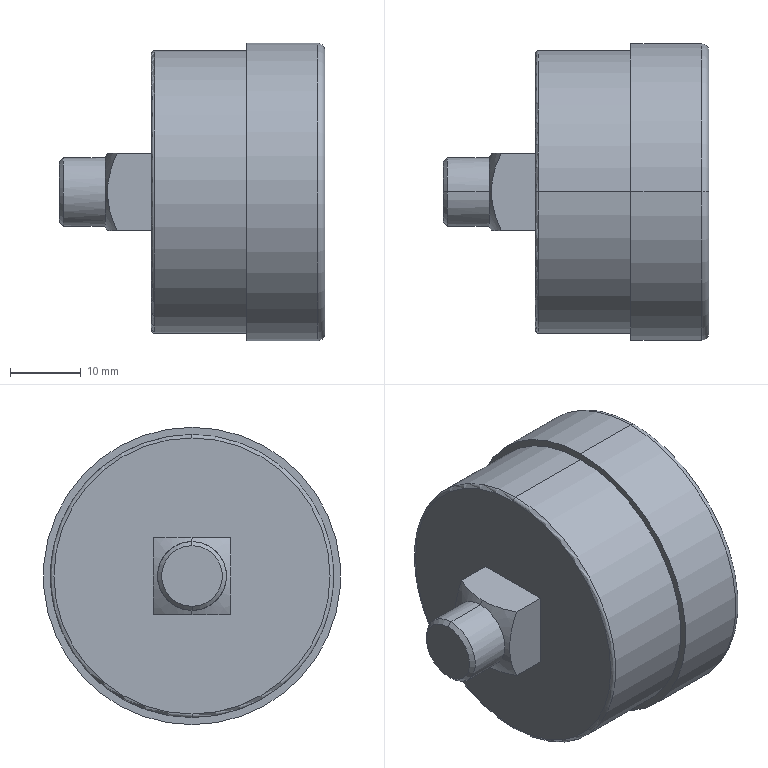Part | SolidWorks | features BaseBody 1 | 1 solid | 25 faces | box 37.5 x 42 x 42 mm | volume 32291 mm3 | plane 9 | cylinder 8 | torus 4 | cone 2 | spline 2 | commonest cylinder face diameters 9.728 x2 37.8 x2 40 x2 42 x2
STEP:
#1=CARTESIAN_POINT('',(-12.419,0.000000001,4.864));
#2=VERTEX_POINT('',#1);
#3=CARTESIAN_POINT('',(-12.419,-0.000000001,-4.864));
#4=VERTEX_POINT('',#3);
#5=CARTESIAN_POINT('',(-12.419,0.,0.));
#6=DIRECTION('',(1.,0.,0.));
#7=DIRECTION('',(0.,0.,-1.));
#8=AXIS2_PLACEMENT_3D('',#5,#6,#7);
#9=CIRCLE('',#8,4.864);
#10=EDGE_CURVE('',#2,#4,#9,.T.);
#11=ORIENTED_EDGE('',*,*,#10,.T.);
#12=CARTESIAN_POINT('',(-6.5,0.,-4.864));
#13=VERTEX_POINT('',#12);
#14=CARTESIAN_POINT('',(23.5,-0.000000004,-4.864));
#15=DIRECTION('',(1.,0.,0.));
#16=VECTOR('',#15,1000.);
#17=LINE('',#14,#16);
#18=EDGE_CURVE('',#4,#13,#17,.T.);
#19=ORIENTED_EDGE('',*,*,#18,.T.);
#20=CARTESIAN_POINT('',(-6.5,0.,4.864));
#21=VERTEX_POINT('',#20);
#22=CARTESIAN_POINT('',(-6.5,0.,4.864));
#23=CARTESIAN_POINT('',(-6.5,-2.547,4.864));
#24=CARTESIAN_POINT('',(-6.5,-5.09,3.281));
#25=CARTESIAN_POINT('',(-6.5,-6.402,0.));
#26=CARTESIAN_POINT('',(-6.5,-5.09,-3.281));
#27=CARTESIAN_POINT('',(-6.5,-2.547,-4.864));
#28=CARTESIAN_POINT('',(-6.5,0.,-4.864));
#29=B_SPLINE_CURVE_WITH_KNOTS('',6,(#22,#23,#24,#25,#26,#27,#28),.UNSPECIFIED.,.F.,.F.,(7,7),(0.,1.),.UNSPECIFIED.);
#30=EDGE_CURVE('',#21,#13,#29,.T.);
#31=ORIENTED_EDGE('',*,*,#30,.F.);
#32=CARTESIAN_POINT('',(23.5,0.000000004,4.864));
#33=DIRECTION('',(1.,0.,0.));
#34=VECTOR('',#33,1000.);
#35=LINE('',#32,#34);
#36=EDGE_CURVE('',#2,#21,#35,.T.);
#37=ORIENTED_EDGE('',*,*,#36,.F.);
#38=EDGE_LOOP('',(#11,#19,#31,#37));
#39=FACE_OUTER_BOUND('',#38,.T.);
#40=CARTESIAN_POINT('',(23.5,0.,0.));
#41=DIRECTION('',(1.,0.,0.));
#42=DIRECTION('',(0.,0.000000001,1.));
#43=AXIS2_PLACEMENT_3D('',#40,#41,#42);
#44=CYLINDRICAL_SURFACE('',#43,4.864);
#45=ADVANCED_FACE('',(#39),#44,.T.);
#46=CARTESIAN_POINT('',(-13.,0.000000001,4.283));
#47=VERTEX_POINT('',#46);
#48=CARTESIAN_POINT('',(-13.,-0.000000001,-4.283));
#49=VERTEX_POINT('',#48);
#50=CARTESIAN_POINT('',(-13.,0.,0.));
#51=DIRECTION('',(1.,0.,0.));
#52=DIRECTION('',(0.,0.,-1.));
#53=AXIS2_PLACEMENT_3D('',#50,#51,#52);
#54=CIRCLE('',#53,4.283);
#55=EDGE_CURVE('',#47,#49,#54,.T.);
#56=ORIENTED_EDGE('',*,*,#55,.T.);
#57=CARTESIAN_POINT('',(-12.419,-0.000000001,-4.864));
#58=DIRECTION('',(0.7071,0.,-0.7071));
#59=VECTOR('',#58,1000.);
#60=LINE('',#57,#59);
#61=EDGE_CURVE('',#49,#4,#60,.T.);
#62=ORIENTED_EDGE('',*,*,#61,.T.);
#63=ORIENTED_EDGE('',*,*,#10,.F.);
#64=CARTESIAN_POINT('',(-12.419,0.000000001,4.864));
#65=DIRECTION('',(0.7071,0.,0.7071));
#66=VECTOR('',#65,1000.);
#67=LINE('',#64,#66);
#68=EDGE_CURVE('',#47,#2,#67,.T.);
#69=ORIENTED_EDGE('',*,*,#68,.F.);
#70=EDGE_LOOP('',(#56,#62,#63,#69));
#71=FACE_OUTER_BOUND('',#70,.T.);
#72=CARTESIAN_POINT('',(-12.419,0.,0.));
#73=DIRECTION('',(1.,0.,0.));
#74=DIRECTION('',(0.,0.,1.));
#75=AXIS2_PLACEMENT_3D('',#72,#73,#74);
#76=CONICAL_SURFACE('',#75,4.864,0.7854);
#77=ADVANCED_FACE('',(#71),#76,.T.);
#78=CARTESIAN_POINT('',(23.5,0.,-18.9));
#79=VERTEX_POINT('',#78);
#80=CARTESIAN_POINT('',(23.5,-0.000000022,18.9));
#81=VERTEX_POINT('',#80);
#82=CARTESIAN_POINT('',(23.5,0.,0.));
#83=DIRECTION('',(1.,0.,0.));
#84=DIRECTION('',(0.,-0.000000001,1.));
#85=AXIS2_PLACEMENT_3D('',#82,#83,#84);
#86=CIRCLE('',#85,18.9);
#87=EDGE_CURVE('',#79,#81,#86,.T.);
#88=ORIENTED_EDGE('',*,*,#87,.F.);
#89=CARTESIAN_POINT('',(24.5,0.,-18.9));
#90=VERTEX_POINT('',#89);
#91=CARTESIAN_POINT('',(23.5,0.,-18.9));
#92=DIRECTION('',(1.,0.,0.));
#93=VECTOR('',#92,1000.);
#94=LINE('',#91,#93);
#95=EDGE_CURVE('',#79,#90,#94,.T.);
#96=ORIENTED_EDGE('',*,*,#95,.T.);
#97=CARTESIAN_POINT('',(24.5,0.,18.9));
#98=VERTEX_POINT('',#97);
#99=CARTESIAN_POINT('',(24.5,0.,0.));
#100=DIRECTION('',(1.,0.,0.));
#101=DIRECTION('',(0.,0.,-1.));
#102=AXIS2_PLACEMENT_3D('',#99,#100,#101);
#103=CIRCLE('',#102,18.9);
#104=EDGE_CURVE('',#90,#98,#103,.T.);
#105=ORIENTED_EDGE('',*,*,#104,.T.);
#106=CARTESIAN_POINT('',(23.5,0.,18.9));
#107=DIRECTION('',(1.,0.,0.));
#108=VECTOR('',#107,1000.);
#109=LINE('',#106,#108);
#110=EDGE_CURVE('',#81,#98,#109,.T.);
#111=ORIENTED_EDGE('',*,*,#110,.F.);
#112=EDGE_LOOP('',(#88,#96,#105,#111));
#113=FACE_OUTER_BOUND('',#112,.T.);
#114=CARTESIAN_POINT('',(23.5,0.,0.));
#115=DIRECTION('',(1.,0.,0.));
#116=DIRECTION('',(0.,0.,1.));
#117=AXIS2_PLACEMENT_3D('',#114,#115,#116);
#118=CYLINDRICAL_SURFACE('',#117,18.9);
#119=ADVANCED_FACE('',(#113),#118,.F.);
#120=CARTESIAN_POINT('',(23.5,0.000000004,21.));
#121=VERTEX_POINT('',#120);
#122=CARTESIAN_POINT('',(23.5,-0.000000004,-21.));
#123=VERTEX_POINT('',#122);
#124=CARTESIAN_POINT('',(23.5,0.,0.));
#125=DIRECTION('',(1.,0.,0.));
#126=DIRECTION('',(0.,0.,-1.));
#127=AXIS2_PLACEMENT_3D('',#124,#125,#126);
#128=CIRCLE('',#127,21.);
#129=EDGE_CURVE('',#121,#123,#128,.T.);
#130=ORIENTED_EDGE('',*,*,#129,.T.);
#131=CARTESIAN_POINT('',(24.5,-0.000000004,-20.));
#132=VERTEX_POINT('',#131);
#133=CARTESIAN_POINT('',(23.5,-0.000000004,-20.));
#134=DIRECTION('',(0.,-1.,0.));
#135=DIRECTION('',(0.,0.,-1.));
#136=AXIS2_PLACEMENT_3D('',#133,#134,#135);
#137=CIRCLE('',#136,1.);
#138=EDGE_CURVE('',#123,#132,#137,.T.);
#139=ORIENTED_EDGE('',*,*,#138,.T.);
#140=CARTESIAN_POINT('',(24.5,0.,20.));
#141=VERTEX_POINT('',#140);
#142=CARTESIAN_POINT('',(24.5,0.,0.));
#143=DIRECTION('',(1.,0.,0.));
#144=DIRECTION('',(0.,0.,1.));
#145=AXIS2_PLACEMENT_3D('',#142,#143,#144);
#146=CIRCLE('',#145,20.);
#147=EDGE_CURVE('',#141,#132,#146,.T.);
#148=ORIENTED_EDGE('',*,*,#147,.F.);
#149=CARTESIAN_POINT('',(23.5,0.000000004,20.));
#150=DIRECTION('',(0.,1.,0.));
#151=DIRECTION('',(0.,0.,1.));
#152=AXIS2_PLACEMENT_3D('',#149,#150,#151);
#153=CIRCLE('',#152,1.);
#154=EDGE_CURVE('',#121,#141,#153,.T.);
#155=ORIENTED_EDGE('',*,*,#154,.F.);
#156=EDGE_LOOP('',(#130,#139,#148,#155));
#157=FACE_OUTER_BOUND('',#156,.T.);
#158=CARTESIAN_POINT('',(23.5,0.,0.));
#159=DIRECTION('',(1.,0.,0.));
#160=DIRECTION('',(0.,0.,1.));
#161=AXIS2_PLACEMENT_3D('',#158,#159,#160);
#162=TOROIDAL_SURFACE('',#161,20.,1.);
#163=ADVANCED_FACE('',(#157),#162,.T.);
#164=CARTESIAN_POINT('',(13.5,0.000000004,21.));
#165=VERTEX_POINT('',#164);
#166=CARTESIAN_POINT('',(13.5,-0.000000004,-21.));
#167=VERTEX_POINT('',#166);
#168=CARTESIAN_POINT('',(13.5,0.,0.));
#169=DIRECTION('',(1.,0.,0.));
#170=DIRECTION('',(0.,0.,-1.));
#171=AXIS2_PLACEMENT_3D('',#168,#169,#170);
#172=CIRCLE('',#171,21.);
#173=EDGE_CURVE('',#165,#167,#172,.T.);
#174=ORIENTED_EDGE('',*,*,#173,.T.);
#175=CARTESIAN_POINT('',(23.5,-0.000000004,-21.));
#176=DIRECTION('',(1.,0.,0.));
#177=VECTOR('',#176,1000.);
#178=LINE('',#175,#177);
#179=EDGE_CURVE('',#167,#123,#178,.T.);
#180=ORIENTED_EDGE('',*,*,#179,.T.);
#181=ORIENTED_EDGE('',*,*,#129,.F.);
#182=CARTESIAN_POINT('',(23.5,0.000000004,21.));
#183=DIRECTION('',(1.,0.,0.));
#184=VECTOR('',#183,1000.);
#185=LINE('',#182,#184);
#186=EDGE_CURVE('',#165,#121,#185,.T.);
#187=ORIENTED_EDGE('',*,*,#186,.F.);
#188=EDGE_LOOP('',(#174,#180,#181,#187));
#189=FACE_OUTER_BOUND('',#188,.T.);
#190=CARTESIAN_POINT('',(23.5,0.,0.));
#191=DIRECTION('',(1.,0.,0.));
#192=DIRECTION('',(0.,0.,1.));
#193=AXIS2_PLACEMENT_3D('',#190,#191,#192);
#194=CYLINDRICAL_SURFACE('',#193,21.);
#195=ADVANCED_FACE('',(#189),#194,.T.);
#196=CARTESIAN_POINT('',(0.5,0.000000023,20.));
#197=VERTEX_POINT('',#196);
#198=CARTESIAN_POINT('',(0.5,-0.000000023,-20.));
#199=VERTEX_POINT('',#198);
#200=CARTESIAN_POINT('',(0.5,0.,0.));
#201=DIRECTION('',(1.,0.,0.));
#202=DIRECTION('',(0.,0.,-1.));
#203=AXIS2_PLACEMENT_3D('',#200,#201,#202);
#204=CIRCLE('',#203,20.);
#205=EDGE_CURVE('',#197,#199,#204,.T.);
#206=ORIENTED_EDGE('',*,*,#205,.T.);
#207=CARTESIAN_POINT('',(13.5,-0.000000015,-20.));
#208=VERTEX_POINT('',#207);
#209=CARTESIAN_POINT('',(23.5,-0.000000015,-20.));
#210=DIRECTION('',(1.,0.,0.));
#211=VECTOR('',#210,1000.);
#212=LINE('',#209,#211);
#213=EDGE_CURVE('',#199,#208,#212,.T.);
#214=ORIENTED_EDGE('',*,*,#213,.T.);
#215=CARTESIAN_POINT('',(13.5,0.,20.));
#216=VERTEX_POINT('',#215);
#217=CARTESIAN_POINT('',(13.5,0.,0.));
#218=DIRECTION('',(1.,0.,0.));
#219=DIRECTION('',(0.,0.,1.));
#220=AXIS2_PLACEMENT_3D('',#217,#218,#219);
#221=CIRCLE('',#220,20.);
#222=EDGE_CURVE('',#216,#208,#221,.T.);
#223=ORIENTED_EDGE('',*,*,#222,.F.);
#224=CARTESIAN_POINT('',(23.5,0.000000015,20.));
#225=DIRECTION('',(1.,0.,0.));
#226=VECTOR('',#225,1000.);
#227=LINE('',#224,#226);
#228=EDGE_CURVE('',#197,#216,#227,.T.);
#229=ORIENTED_EDGE('',*,*,#228,.F.);
#230=EDGE_LOOP('',(#206,#214,#223,#229));
#231=FACE_OUTER_BOUND('',#230,.T.);
#232=CARTESIAN_POINT('',(23.5,0.,0.));
#233=DIRECTION('',(1.,0.,0.));
#234=DIRECTION('',(0.,0.000000001,1.));
#235=AXIS2_PLACEMENT_3D('',#232,#233,#234);
#236=CYLINDRICAL_SURFACE('',#235,20.);
#237=ADVANCED_FACE('',(#231),#236,.T.);
#238=CARTESIAN_POINT('',(0.,0.000000023,19.5));
#239=VERTEX_POINT('',#238);
#240=CARTESIAN_POINT('',(0.,-0.000000023,-19.5));
#241=VERTEX_POINT('',#240);
#242=CARTESIAN_POINT('',(0.,0.,0.));
#243=DIRECTION('',(1.,0.,0.));
#244=DIRECTION('',(0.,0.,-1.));
#245=AXIS2_PLACEMENT_3D('',#242,#243,#244);
#246=CIRCLE('',#245,19.5);
#247=EDGE_CURVE('',#239,#241,#246,.T.);
#248=ORIENTED_EDGE('',*,*,#247,.T.);
#249=CARTESIAN_POINT('',(0.5,-0.000000023,-19.5));
#250=DIRECTION('',(0.,-1.,0.000000001));
#251=DIRECTION('',(0.,-0.000000001,-1.));
#252=AXIS2_PLACEMENT_3D('',#249,#250,#251);
#253=CIRCLE('',#252,0.5);
#254=EDGE_CURVE('',#241,#199,#253,.T.);
#255=ORIENTED_EDGE('',*,*,#254,.T.);
#256=ORIENTED_EDGE('',*,*,#205,.F.);
#257=CARTESIAN_POINT('',(0.5,0.000000023,19.5));
#258=DIRECTION('',(0.,1.,-0.000000001));
#259=DIRECTION('',(0.,0.000000001,1.));
#260=AXIS2_PLACEMENT_3D('',#257,#258,#259);
#261=CIRCLE('',#260,0.5);
#262=EDGE_CURVE('',#239,#197,#261,.T.);
#263=ORIENTED_EDGE('',*,*,#262,.F.);
#264=EDGE_LOOP('',(#248,#255,#256,#263));
#265=FACE_OUTER_BOUND('',#264,.T.);
#266=CARTESIAN_POINT('',(0.5,0.,0.));
#267=DIRECTION('',(1.,0.,0.));
#268=DIRECTION('',(0.,0.000000001,1.));
#269=AXIS2_PLACEMENT_3D('',#266,#267,#268);
#270=TOROIDAL_SURFACE('',#269,19.5,0.5);
#271=ADVANCED_FACE('',(#265),#270,.T.);
#272=ORIENTED_EDGE('',*,*,#247,.F.);
#273=CARTESIAN_POINT('',(0.,0.,0.));
#274=DIRECTION('',(1.,0.,0.));
#275=DIRECTION('',(0.,0.,-1.));
#276=AXIS2_PLACEMENT_3D('',#273,#274,#275);
#277=CIRCLE('',#276,19.5);
#278=EDGE_CURVE('',#241,#239,#277,.T.);
#279=ORIENTED_EDGE('',*,*,#278,.F.);
#280=EDGE_LOOP('',(#272,#279));
#281=FACE_OUTER_BOUND('',#280,.T.);
#282=CARTESIAN_POINT('',(0.,5.5,5.5));
#283=VERTEX_POINT('',#282);
#284=CARTESIAN_POINT('',(0.,-5.5,5.5));
#285=VERTEX_POINT('',#284);
#286=CARTESIAN_POINT('',(0.,5.5,5.5));
#287=DIRECTION('',(0.,-1.,0.));
#288=VECTOR('',#287,1000.);
#289=LINE('',#286,#288);
#290=EDGE_CURVE('',#283,#285,#289,.T.);
#291=ORIENTED_EDGE('',*,*,#290,.T.);
#292=CARTESIAN_POINT('',(0.,-5.5,-5.5));
#293=VERTEX_POINT('',#292);
#294=CARTESIAN_POINT('',(0.,-5.5,5.5));
#295=DIRECTION('',(0.,0.,-1.));
#296=VECTOR('',#295,1000.);
#297=LINE('',#294,#296);
#298=EDGE_CURVE('',#285,#293,#297,.T.);
#299=ORIENTED_EDGE('',*,*,#298,.T.);
#300=CARTESIAN_POINT('',(0.,5.5,-5.5));
#301=VERTEX_POINT('',#300);
#302=CARTESIAN_POINT('',(0.,-5.5,-5.5));
#303=DIRECTION('',(0.,1.,0.));
#304=VECTOR('',#303,1000.);
#305=LINE('',#302,#304);
#306=EDGE_CURVE('',#293,#301,#305,.T.);
#307=ORIENTED_EDGE('',*,*,#306,.T.);
#308=CARTESIAN_POINT('',(0.,5.5,-5.5));
#309=DIRECTION('',(0.,0.,1.));
#310=VECTOR('',#309,1000.);
#311=LINE('',#308,#310);
#312=EDGE_CURVE('',#301,#283,#311,.T.);
#313=ORIENTED_EDGE('',*,*,#312,.T.);
#314=EDGE_LOOP('',(#291,#299,#307,#313));
#315=FACE_BOUND('',#314,.T.);
#316=CARTESIAN_POINT('',(0.,-19.862,19.5));
#317=DIRECTION('',(-1.,0.,0.));
#318=DIRECTION('',(0.,1.,0.));
#319=AXIS2_PLACEMENT_3D('',#316,#317,#318);
#320=PLANE('',#319);
#321=ADVANCED_FACE('',(#281,#315),#320,.T.);
#322=ORIENTED_EDGE('',*,*,#173,.F.);
#323=CARTESIAN_POINT('',(13.5,0.,0.));
#324=DIRECTION('',(1.,0.,0.));
#325=DIRECTION('',(0.,0.,-1.));
#326=AXIS2_PLACEMENT_3D('',#323,#324,#325);
#327=CIRCLE('',#326,21.);
#328=EDGE_CURVE('',#167,#165,#327,.T.);
#329=ORIENTED_EDGE('',*,*,#328,.F.);
#330=EDGE_LOOP('',(#322,#329));
#331=FACE_OUTER_BOUND('',#330,.T.);
#332=ORIENTED_EDGE('',*,*,#222,.T.);
#333=CARTESIAN_POINT('',(13.5,0.,0.));
#334=DIRECTION('',(1.,0.,0.));
#335=DIRECTION('',(0.,0.,1.));
#336=AXIS2_PLACEMENT_3D('',#333,#334,#335);
#337=CIRCLE('',#336,20.);
#338=EDGE_CURVE('',#208,#216,#337,.T.);
#339=ORIENTED_EDGE('',*,*,#338,.T.);
#340=EDGE_LOOP('',(#332,#339));
#341=FACE_BOUND('',#340,.T.);
#342=CARTESIAN_POINT('',(13.5,-21.39,21.));
#343=DIRECTION('',(-1.,0.,0.));
#344=DIRECTION('',(0.,1.,0.));
#345=AXIS2_PLACEMENT_3D('',#342,#343,#344);
#346=PLANE('',#345);
#347=ADVANCED_FACE('',(#331,#341),#346,.T.);
#348=ORIENTED_EDGE('',*,*,#147,.T.);
#349=CARTESIAN_POINT('',(24.5,0.,0.));
#350=DIRECTION('',(1.,0.,0.));
#351=DIRECTION('',(0.,0.,1.));
#352=AXIS2_PLACEMENT_3D('',#349,#350,#351);
#353=CIRCLE('',#352,20.);
#354=EDGE_CURVE('',#132,#141,#353,.T.);
#355=ORIENTED_EDGE('',*,*,#354,.T.);
#356=EDGE_LOOP('',(#348,#355));
#357=FACE_OUTER_BOUND('',#356,.T.);
#358=CARTESIAN_POINT('',(24.5,0.,0.));
#359=DIRECTION('',(1.,0.,0.));
#360=DIRECTION('',(0.,0.,-1.));
#361=AXIS2_PLACEMENT_3D('',#358,#359,#360);
#362=CIRCLE('',#361,18.9);
#363=EDGE_CURVE('',#98,#90,#362,.T.);
#364=ORIENTED_EDGE('',*,*,#363,.F.);
#365=ORIENTED_EDGE('',*,*,#104,.F.);
#366=EDGE_LOOP('',(#364,#365));
#367=FACE_BOUND('',#366,.T.);
#368=CARTESIAN_POINT('',(24.5,-20.372,-20.));
#369=DIRECTION('',(1.,0.,0.));
#370=DIRECTION('',(0.,1.,0.));
#371=AXIS2_PLACEMENT_3D('',#368,#369,#370);
#372=PLANE('',#371);
#373=ADVANCED_FACE('',(#357,#367),#372,.T.);
#374=CARTESIAN_POINT('',(23.5,0.,0.));
#375=DIRECTION('',(1.,0.,0.));
#376=DIRECTION('',(0.,-0.000000001,1.));
#377=AXIS2_PLACEMENT_3D('',#374,#375,#376);
#378=CIRCLE('',#377,18.9);
#379=EDGE_CURVE('',#81,#79,#378,.T.);
#380=ORIENTED_EDGE('',*,*,#379,.T.);
#381=ORIENTED_EDGE('',*,*,#87,.T.);
#382=EDGE_LOOP('',(#380,#381));
#383=FACE_OUTER_BOUND('',#382,.T.);
#384=CARTESIAN_POINT('',(23.5,-19.251,-18.9));
#385=DIRECTION('',(1.,0.,0.));
#386=DIRECTION('',(0.,1.,0.));
#387=AXIS2_PLACEMENT_3D('',#384,#385,#386);
#388=PLANE('',#387);
#389=ADVANCED_FACE('',(#383),#388,.T.);
#390=CARTESIAN_POINT('',(-4.806,-5.5,5.5));
#391=VERTEX_POINT('',#390);
#392=CARTESIAN_POINT('',(-4.806,-5.5,5.5));
#393=DIRECTION('',(1.,0.000007521,0.));
#394=VECTOR('',#393,1000.);
#395=LINE('',#392,#394);
#396=EDGE_CURVE('',#391,#285,#395,.T.);
#397=ORIENTED_EDGE('',*,*,#396,.T.);
#398=ORIENTED_EDGE('',*,*,#290,.F.);
#399=CARTESIAN_POINT('',(-4.806,5.5,5.5));
#400=VERTEX_POINT('',#399);
#401=CARTESIAN_POINT('',(0.,5.5,5.5));
#402=DIRECTION('',(1.,0.000000001,0.));
#403=VECTOR('',#402,1000.);
#404=LINE('',#401,#403);
#405=EDGE_CURVE('',#400,#283,#404,.T.);
#406=ORIENTED_EDGE('',*,*,#405,.F.);
#407=CARTESIAN_POINT('',(-6.185,0.,5.5));
#408=VERTEX_POINT('',#407);
#409=CARTESIAN_POINT('',(-6.185,0.,5.5));
#410=CARTESIAN_POINT('',(-6.185,0.1878,5.5));
#411=CARTESIAN_POINT('',(-6.18,0.3546,5.5));
#412=CARTESIAN_POINT('',(-6.165,0.6789,5.5));
#413=CARTESIAN_POINT('',(-6.153,0.8322,5.5));
#414=CARTESIAN_POINT('',(-6.114,1.261,5.5));
#415=CARTESIAN_POINT('',(-6.082,1.505,5.5));
#416=CARTESIAN_POINT('',(-6.004,1.984,5.5));
#417=CARTESIAN_POINT('',(-5.96,2.211,5.5));
#418=CARTESIAN_POINT('',(-5.86,2.654,5.5));
#419=CARTESIAN_POINT('',(-5.803,2.877,5.5));
#420=CARTESIAN_POINT('',(-5.681,3.309,5.5));
#421=CARTESIAN_POINT('',(-5.615,3.519,5.5));
#422=CARTESIAN_POINT('',(-5.478,3.924,5.5));
#423=CARTESIAN_POINT('',(-5.407,4.119,5.5));
#424=CARTESIAN_POINT('',(-5.186,4.685,5.499));
#425=CARTESIAN_POINT('',(-5.015,5.078,5.5));
#426=CARTESIAN_POINT('',(-4.806,5.5,5.5));
#427=B_SPLINE_CURVE_WITH_KNOTS('',3,(#409,#410,#411,#412,#413,#414,#415,#416,#417,#418,#419,#420,#421,#422,#423,#424,#425,#426),.UNSPECIFIED.,.F.,.F.,(4,2,2,2,2,2,2,2,4),(0.,0.0625,0.125,0.25,0.375,0.5,0.625,0.75,1.),.UNSPECIFIED.);
#428=EDGE_CURVE('',#408,#400,#427,.T.);
#429=ORIENTED_EDGE('',*,*,#428,.F.);
#430=CARTESIAN_POINT('',(-4.806,-5.5,5.5));
#431=CARTESIAN_POINT('',(-5.044,-5.019,5.5));
#432=CARTESIAN_POINT('',(-5.237,-4.571,5.499));
#433=CARTESIAN_POINT('',(-5.449,-4.001,5.5));
#434=CARTESIAN_POINT('',(-5.49,-3.886,5.5));
#435=CARTESIAN_POINT('',(-5.568,-3.66,5.5));
#436=CARTESIAN_POINT('',(-5.604,-3.549,5.5));
#437=CARTESIAN_POINT('',(-5.707,-3.221,5.5));
#438=CARTESIAN_POINT('',(-5.767,-3.009,5.5));
#439=CARTESIAN_POINT('',(-5.875,-2.59,5.5));
#440=CARTESIAN_POINT('',(-5.923,-2.382,5.5));
#441=CARTESIAN_POINT('',(-5.987,-2.061,5.5));
#442=CARTESIAN_POINT('',(-6.008,-1.952,5.5));
#443=CARTESIAN_POINT('',(-6.045,-1.735,5.5));
#444=CARTESIAN_POINT('',(-6.062,-1.626,5.5));
#445=CARTESIAN_POINT('',(-6.093,-1.403,5.5));
#446=CARTESIAN_POINT('',(-6.108,-1.29,5.5));
#447=CARTESIAN_POINT('',(-6.134,-1.052,5.5));
#448=CARTESIAN_POINT('',(-6.145,-0.9281,5.5));
#449=CARTESIAN_POINT('',(-6.174,-0.5463,5.5));
#450=CARTESIAN_POINT('',(-6.185,-0.2841,5.5));
#451=CARTESIAN_POINT('',(-6.185,0.,5.5));
#452=B_SPLINE_CURVE_WITH_KNOTS('',3,(#430,#431,#432,#433,#434,#435,#436,#437,#438,#439,#440,#441,#442,#443,#444,#445,#446,#447,#448,#449,#450,#451),.UNSPECIFIED.,.F.,.F.,(4,2,2,2,2,2,2,2,2,2,4),(0.,0.25,0.3125,0.375,0.5,0.625,0.6875,0.75,0.8125,0.875,1.),.UNSPECIFIED.);
#453=EDGE_CURVE('',#391,#408,#452,.T.);
#454=ORIENTED_EDGE('',*,*,#453,.F.);
#455=EDGE_LOOP('',(#397,#398,#406,#429,#454));
#456=FACE_OUTER_BOUND('',#455,.T.);
#457=CARTESIAN_POINT('',(-6.185,-5.5,5.5));
#458=DIRECTION('',(0.,0.,1.));
#459=DIRECTION('',(1.,0.,0.));
#460=AXIS2_PLACEMENT_3D('',#457,#458,#459);
#461=PLANE('',#460);
#462=ADVANCED_FACE('',(#456),#461,.T.);
#463=ORIENTED_EDGE('',*,*,#405,.T.);
#464=ORIENTED_EDGE('',*,*,#312,.F.);
#465=CARTESIAN_POINT('',(-4.806,5.5,-5.5));
#466=VERTEX_POINT('',#465);
#467=CARTESIAN_POINT('',(0.,5.5,-5.5));
#468=DIRECTION('',(1.,0.,-0.000000001));
#469=VECTOR('',#468,1000.);
#470=LINE('',#467,#469);
#471=EDGE_CURVE('',#466,#301,#470,.T.);
#472=ORIENTED_EDGE('',*,*,#471,.F.);
#473=CARTESIAN_POINT('',(-4.806,5.5,5.5));
#474=CARTESIAN_POINT('',(-5.066,5.5,4.975));
#475=CARTESIAN_POINT('',(-5.272,5.499,4.488));
#476=CARTESIAN_POINT('',(-5.498,5.5,3.864));
#477=CARTESIAN_POINT('',(-5.541,5.5,3.739));
#478=CARTESIAN_POINT('',(-5.621,5.5,3.496));
#479=CARTESIAN_POINT('',(-5.658,5.5,3.377));
#480=CARTESIAN_POINT('',(-5.763,5.5,3.024));
#481=CARTESIAN_POINT('',(-5.824,5.5,2.795));
#482=CARTESIAN_POINT('',(-5.905,5.5,2.453));
#483=CARTESIAN_POINT('',(-5.931,5.5,2.338));
#484=CARTESIAN_POINT('',(-5.978,5.5,2.106));
#485=CARTESIAN_POINT('',(-6.001,5.5,1.986));
#486=CARTESIAN_POINT('',(-6.063,5.5,1.631));
#487=CARTESIAN_POINT('',(-6.097,5.5,1.394));
#488=CARTESIAN_POINT('',(-6.139,5.5,1.001));
#489=CARTESIAN_POINT('',(-6.151,5.5,0.8644));
#490=CARTESIAN_POINT('',(-6.165,5.5,0.6525));
#491=CARTESIAN_POINT('',(-6.169,5.5,0.5801));
#492=CARTESIAN_POINT('',(-6.177,5.5,0.4282));
#493=CARTESIAN_POINT('',(-6.179,5.5,0.3474));
#494=CARTESIAN_POINT('',(-6.186,5.5,0.1074));
#495=CARTESIAN_POINT('',(-6.186,5.5,-0.05478));
#496=CARTESIAN_POINT('',(-6.18,5.5,-0.3746));
#497=CARTESIAN_POINT('',(-6.173,5.5,-0.5188));
#498=CARTESIAN_POINT('',(-6.147,5.5,-0.9397));
#499=CARTESIAN_POINT('',(-6.122,5.5,-1.181));
#500=CARTESIAN_POINT('',(-6.077,5.5,-1.521));
#501=CARTESIAN_POINT('',(-6.061,5.5,-1.631));
#502=CARTESIAN_POINT('',(-6.026,5.5,-1.847));
#503=CARTESIAN_POINT('',(-6.007,5.5,-1.955));
#504=CARTESIAN_POINT('',(-5.947,5.5,-2.269));
#505=CARTESIAN_POINT('',(-5.902,5.5,-2.471));
#506=CARTESIAN_POINT('',(-5.802,5.5,-2.879));
#507=CARTESIAN_POINT('',(-5.746,5.5,-3.083));
#508=CARTESIAN_POINT('',(-5.628,5.5,-3.476));
#509=CARTESIAN_POINT('',(-5.566,5.5,-3.667));
#510=CARTESIAN_POINT('',(-5.437,5.5,-4.037));
#511=CARTESIAN_POINT('',(-5.371,5.5,-4.212));
#512=CARTESIAN_POINT('',(-5.161,5.499,-4.744));
#513=CARTESIAN_POINT('',(-4.999,5.5,-5.109));
#514=CARTESIAN_POINT('',(-4.806,5.5,-5.5));
#515=B_SPLINE_CURVE_WITH_KNOTS('',3,(#473,#474,#475,#476,#477,#478,#479,#480,#481,#482,#483,#484,#485,#486,#487,#488,#489,#490,#491,#492,#493,#494,#495,#496,#497,#498,#499,#500,#501,#502,#503,#504,#505,#506,#507,#508,#509,#510,#511,#512,#513,#514),.UNSPECIFIED.,.F.,.F.,(4,2,2,2,2,2,2,2,2,2,2,2,2,2,2,2,2,2,2,2,4),(0.,0.125,0.1563,0.1875,0.25,0.2813,0.3125,0.375,0.4063,0.4219,0.4375,0.4688,0.5,0.5625,0.5938,0.625,0.6875,0.75,0.8125,0.875,1.),.UNSPECIFIED.);
#516=EDGE_CURVE('',#400,#466,#515,.T.);
#517=ORIENTED_EDGE('',*,*,#516,.F.);
#518=EDGE_LOOP('',(#463,#464,#472,#517));
#519=FACE_OUTER_BOUND('',#518,.T.);
#520=CARTESIAN_POINT('',(-6.204,5.5,-5.5));
#521=DIRECTION('',(0.,1.,0.));
#522=DIRECTION('',(0.,0.,1.));
#523=AXIS2_PLACEMENT_3D('',#520,#521,#522);
#524=PLANE('',#523);
#525=ADVANCED_FACE('',(#519),#524,.T.);
#526=ORIENTED_EDGE('',*,*,#471,.T.);
#527=ORIENTED_EDGE('',*,*,#306,.F.);
#528=CARTESIAN_POINT('',(-4.806,-5.5,-5.5));
#529=VERTEX_POINT('',#528);
#530=CARTESIAN_POINT('',(0.,-5.5,-5.5));
#531=DIRECTION('',(1.,-0.000000001,0.));
#532=VECTOR('',#531,1000.);
#533=LINE('',#530,#532);
#534=EDGE_CURVE('',#529,#293,#533,.T.);
#535=ORIENTED_EDGE('',*,*,#534,.F.);
#536=CARTESIAN_POINT('',(-6.185,0.,-5.5));
#537=VERTEX_POINT('',#536);
#538=CARTESIAN_POINT('',(-6.185,0.,-5.5));
#539=CARTESIAN_POINT('',(-6.185,-0.1878,-5.5));
#540=CARTESIAN_POINT('',(-6.18,-0.3546,-5.5));
#541=CARTESIAN_POINT('',(-6.165,-0.6789,-5.5));
#542=CARTESIAN_POINT('',(-6.153,-0.8322,-5.5));
#543=CARTESIAN_POINT('',(-6.114,-1.261,-5.5));
#544=CARTESIAN_POINT('',(-6.082,-1.505,-5.5));
#545=CARTESIAN_POINT('',(-6.004,-1.984,-5.5));
#546=CARTESIAN_POINT('',(-5.96,-2.211,-5.5));
#547=CARTESIAN_POINT('',(-5.86,-2.654,-5.5));
#548=CARTESIAN_POINT('',(-5.803,-2.877,-5.5));
#549=CARTESIAN_POINT('',(-5.681,-3.309,-5.5));
#550=CARTESIAN_POINT('',(-5.615,-3.519,-5.5));
#551=CARTESIAN_POINT('',(-5.478,-3.924,-5.5));
#552=CARTESIAN_POINT('',(-5.407,-4.119,-5.5));
#553=CARTESIAN_POINT('',(-5.186,-4.685,-5.499));
#554=CARTESIAN_POINT('',(-5.015,-5.078,-5.5));
#555=CARTESIAN_POINT('',(-4.806,-5.5,-5.5));
#556=B_SPLINE_CURVE_WITH_KNOTS('',3,(#538,#539,#540,#541,#542,#543,#544,#545,#546,#547,#548,#549,#550,#551,#552,#553,#554,#555),.UNSPECIFIED.,.F.,.F.,(4,2,2,2,2,2,2,2,4),(0.,0.0625,0.125,0.25,0.375,0.5,0.625,0.75,1.),.UNSPECIFIED.);
#557=EDGE_CURVE('',#537,#529,#556,.T.);
#558=ORIENTED_EDGE('',*,*,#557,.F.);
#559=CARTESIAN_POINT('',(-4.806,5.5,-5.5));
#560=CARTESIAN_POINT('',(-5.044,5.019,-5.5));
#561=CARTESIAN_POINT('',(-5.237,4.571,-5.499));
#562=CARTESIAN_POINT('',(-5.449,4.001,-5.5));
#563=CARTESIAN_POINT('',(-5.49,3.886,-5.5));
#564=CARTESIAN_POINT('',(-5.568,3.66,-5.5));
#565=CARTESIAN_POINT('',(-5.604,3.549,-5.5));
#566=CARTESIAN_POINT('',(-5.707,3.221,-5.5));
#567=CARTESIAN_POINT('',(-5.767,3.009,-5.5));
#568=CARTESIAN_POINT('',(-5.875,2.59,-5.5));
#569=CARTESIAN_POINT('',(-5.923,2.382,-5.5));
#570=CARTESIAN_POINT('',(-5.987,2.061,-5.5));
#571=CARTESIAN_POINT('',(-6.008,1.952,-5.5));
#572=CARTESIAN_POINT('',(-6.045,1.735,-5.5));
#573=CARTESIAN_POINT('',(-6.062,1.626,-5.5));
#574=CARTESIAN_POINT('',(-6.093,1.403,-5.5));
#575=CARTESIAN_POINT('',(-6.108,1.29,-5.5));
#576=CARTESIAN_POINT('',(-6.134,1.052,-5.5));
#577=CARTESIAN_POINT('',(-6.145,0.9281,-5.5));
#578=CARTESIAN_POINT('',(-6.174,0.5463,-5.5));
#579=CARTESIAN_POINT('',(-6.185,0.2841,-5.5));
#580=CARTESIAN_POINT('',(-6.185,0.,-5.5));
#581=B_SPLINE_CURVE_WITH_KNOTS('',3,(#559,#560,#561,#562,#563,#564,#565,#566,#567,#568,#569,#570,#571,#572,#573,#574,#575,#576,#577,#578,#579,#580),.UNSPECIFIED.,.F.,.F.,(4,2,2,2,2,2,2,2,2,2,4),(0.,0.25,0.3125,0.375,0.5,0.625,0.6875,0.75,0.8125,0.875,1.),.UNSPECIFIED.);
#582=EDGE_CURVE('',#466,#537,#581,.T.);
#583=ORIENTED_EDGE('',*,*,#582,.F.);
#584=EDGE_LOOP('',(#526,#527,#535,#558,#583));
#585=FACE_OUTER_BOUND('',#584,.T.);
#586=CARTESIAN_POINT('',(0.,-5.5,-5.5));
#587=DIRECTION('',(0.,0.,-1.));
#588=DIRECTION('',(-1.,0.,0.));
#589=AXIS2_PLACEMENT_3D('',#586,#587,#588);
#590=PLANE('',#589);
#591=ADVANCED_FACE('',(#585),#590,.T.);
#592=ORIENTED_EDGE('',*,*,#534,.T.);
#593=ORIENTED_EDGE('',*,*,#298,.F.);
#594=ORIENTED_EDGE('',*,*,#396,.F.);
#595=CARTESIAN_POINT('',(-4.806,-5.5,-5.5));
#596=CARTESIAN_POINT('',(-5.066,-5.5,-4.975));
#597=CARTESIAN_POINT('',(-5.272,-5.499,-4.488));
#598=CARTESIAN_POINT('',(-5.498,-5.5,-3.864));
#599=CARTESIAN_POINT('',(-5.541,-5.5,-3.739));
#600=CARTESIAN_POINT('',(-5.621,-5.5,-3.496));
#601=CARTESIAN_POINT('',(-5.658,-5.5,-3.377));
#602=CARTESIAN_POINT('',(-5.763,-5.5,-3.024));
#603=CARTESIAN_POINT('',(-5.824,-5.5,-2.795));
#604=CARTESIAN_POINT('',(-5.905,-5.5,-2.453));
#605=CARTESIAN_POINT('',(-5.931,-5.5,-2.338));
#606=CARTESIAN_POINT('',(-5.978,-5.5,-2.106));
#607=CARTESIAN_POINT('',(-6.001,-5.5,-1.986));
#608=CARTESIAN_POINT('',(-6.063,-5.5,-1.631));
#609=CARTESIAN_POINT('',(-6.097,-5.5,-1.394));
#610=CARTESIAN_POINT('',(-6.139,-5.5,-1.001));
#611=CARTESIAN_POINT('',(-6.151,-5.5,-0.8644));
#612=CARTESIAN_POINT('',(-6.165,-5.5,-0.6525));
#613=CARTESIAN_POINT('',(-6.169,-5.5,-0.5801));
#614=CARTESIAN_POINT('',(-6.177,-5.5,-0.4282));
#615=CARTESIAN_POINT('',(-6.179,-5.5,-0.3474));
#616=CARTESIAN_POINT('',(-6.186,-5.5,-0.1074));
#617=CARTESIAN_POINT('',(-6.186,-5.5,0.05478));
#618=CARTESIAN_POINT('',(-6.18,-5.5,0.3746));
#619=CARTESIAN_POINT('',(-6.173,-5.5,0.5188));
#620=CARTESIAN_POINT('',(-6.147,-5.5,0.9397));
#621=CARTESIAN_POINT('',(-6.122,-5.5,1.181));
#622=CARTESIAN_POINT('',(-6.077,-5.5,1.521));
#623=CARTESIAN_POINT('',(-6.061,-5.5,1.631));
#624=CARTESIAN_POINT('',(-6.026,-5.5,1.847));
#625=CARTESIAN_POINT('',(-6.007,-5.5,1.955));
#626=CARTESIAN_POINT('',(-5.947,-5.5,2.269));
#627=CARTESIAN_POINT('',(-5.902,-5.5,2.471));
#628=CARTESIAN_POINT('',(-5.802,-5.5,2.879));
#629=CARTESIAN_POINT('',(-5.746,-5.5,3.083));
#630=CARTESIAN_POINT('',(-5.628,-5.5,3.476));
#631=CARTESIAN_POINT('',(-5.566,-5.5,3.667));
#632=CARTESIAN_POINT('',(-5.437,-5.5,4.037));
#633=CARTESIAN_POINT('',(-5.371,-5.5,4.212));
#634=CARTESIAN_POINT('',(-5.161,-5.499,4.744));
#635=CARTESIAN_POINT('',(-4.999,-5.5,5.109));
#636=CARTESIAN_POINT('',(-4.806,-5.5,5.5));
#637=B_SPLINE_CURVE_WITH_KNOTS('',3,(#595,#596,#597,#598,#599,#600,#601,#602,#603,#604,#605,#606,#607,#608,#609,#610,#611,#612,#613,#614,#615,#616,#617,#618,#619,#620,#621,#622,#623,#624,#625,#626,#627,#628,#629,#630,#631,#632,#633,#634,#635,#636),.UNSPECIFIED.,.F.,.F.,(4,2,2,2,2,2,2,2,2,2,2,2,2,2,2,2,2,2,2,2,4),(0.,0.125,0.1562,0.1875,0.25,0.2812,0.3125,0.375,0.4063,0.4219,0.4375,0.4688,0.5,0.5625,0.5938,0.625,0.6875,0.75,0.8125,0.875,1.),.UNSPECIFIED.);
#638=EDGE_CURVE('',#529,#391,#637,.T.);
#639=ORIENTED_EDGE('',*,*,#638,.F.);
#640=EDGE_LOOP('',(#592,#593,#594,#639));
#641=FACE_OUTER_BOUND('',#640,.T.);
#642=CARTESIAN_POINT('',(-6.204,-5.5,5.5));
#643=DIRECTION('',(0.,-1.,0.));
#644=DIRECTION('',(0.,0.,-1.));
#645=AXIS2_PLACEMENT_3D('',#642,#643,#644);
#646=PLANE('',#645);
#647=ADVANCED_FACE('',(#641),#646,.T.);
#648=ORIENTED_EDGE('',*,*,#55,.F.);
#649=CARTESIAN_POINT('',(-13.,0.,0.));
#650=DIRECTION('',(1.,0.,0.));
#651=DIRECTION('',(0.,0.,-1.));
#652=AXIS2_PLACEMENT_3D('',#649,#650,#651);
#653=CIRCLE('',#652,4.283);
#654=EDGE_CURVE('',#49,#47,#653,.T.);
#655=ORIENTED_EDGE('',*,*,#654,.F.);
#656=EDGE_LOOP('',(#648,#655));
#657=FACE_OUTER_BOUND('',#656,.T.);
#658=CARTESIAN_POINT('',(-13.,-4.283,4.283));
#659=DIRECTION('',(-1.,0.,0.));
#660=DIRECTION('',(0.,1.,0.));
#661=AXIS2_PLACEMENT_3D('',#658,#659,#660);
#662=PLANE('',#661);
#663=ADVANCED_FACE('',(#657),#662,.T.);
#664=ORIENTED_EDGE('',*,*,#254,.F.);
#665=ORIENTED_EDGE('',*,*,#278,.T.);
#666=ORIENTED_EDGE('',*,*,#262,.T.);
#667=CARTESIAN_POINT('',(0.5,0.,0.));
#668=DIRECTION('',(1.,0.,0.));
#669=DIRECTION('',(0.,0.,-1.));
#670=AXIS2_PLACEMENT_3D('',#667,#668,#669);
#671=CIRCLE('',#670,20.);
#672=EDGE_CURVE('',#199,#197,#671,.T.);
#673=ORIENTED_EDGE('',*,*,#672,.F.);
#674=EDGE_LOOP('',(#664,#665,#666,#673));
#675=FACE_OUTER_BOUND('',#674,.T.);
#676=CARTESIAN_POINT('',(0.5,0.,0.));
#677=DIRECTION('',(1.,0.,0.));
#678=DIRECTION('',(0.,0.000000001,1.));
#679=AXIS2_PLACEMENT_3D('',#676,#677,#678);
#680=TOROIDAL_SURFACE('',#679,19.5,0.5);
#681=ADVANCED_FACE('',(#675),#680,.T.);
#682=ORIENTED_EDGE('',*,*,#213,.F.);
#683=ORIENTED_EDGE('',*,*,#672,.T.);
#684=ORIENTED_EDGE('',*,*,#228,.T.);
#685=ORIENTED_EDGE('',*,*,#338,.F.);
#686=EDGE_LOOP('',(#682,#683,#684,#685));
#687=FACE_OUTER_BOUND('',#686,.T.);
#688=CARTESIAN_POINT('',(23.5,0.,0.));
#689=DIRECTION('',(1.,0.,0.));
#690=DIRECTION('',(0.,0.000000001,1.));
#691=AXIS2_PLACEMENT_3D('',#688,#689,#690);
#692=CYLINDRICAL_SURFACE('',#691,20.);
#693=ADVANCED_FACE('',(#687),#692,.T.);
#694=ORIENTED_EDGE('',*,*,#179,.F.);
#695=ORIENTED_EDGE('',*,*,#328,.T.);
#696=ORIENTED_EDGE('',*,*,#186,.T.);
#697=CARTESIAN_POINT('',(23.5,0.,0.));
#698=DIRECTION('',(1.,0.,0.));
#699=DIRECTION('',(0.,0.,-1.));
#700=AXIS2_PLACEMENT_3D('',#697,#698,#699);
#701=CIRCLE('',#700,21.);
#702=EDGE_CURVE('',#123,#121,#701,.T.);
#703=ORIENTED_EDGE('',*,*,#702,.F.);
#704=EDGE_LOOP('',(#694,#695,#696,#703));
#705=FACE_OUTER_BOUND('',#704,.T.);
#706=CARTESIAN_POINT('',(23.5,0.,0.));
#707=DIRECTION('',(1.,0.,0.));
#708=DIRECTION('',(0.,0.,1.));
#709=AXIS2_PLACEMENT_3D('',#706,#707,#708);
#710=CYLINDRICAL_SURFACE('',#709,21.);
#711=ADVANCED_FACE('',(#705),#710,.T.);
#712=ORIENTED_EDGE('',*,*,#138,.F.);
#713=ORIENTED_EDGE('',*,*,#702,.T.);
#714=ORIENTED_EDGE('',*,*,#154,.T.);
#715=ORIENTED_EDGE('',*,*,#354,.F.);
#716=EDGE_LOOP('',(#712,#713,#714,#715));
#717=FACE_OUTER_BOUND('',#716,.T.);
#718=CARTESIAN_POINT('',(23.5,0.,0.));
#719=DIRECTION('',(1.,0.,0.));
#720=DIRECTION('',(0.,0.,1.));
#721=AXIS2_PLACEMENT_3D('',#718,#719,#720);
#722=TOROIDAL_SURFACE('',#721,20.,1.);
#723=ADVANCED_FACE('',(#717),#722,.T.);
#724=ORIENTED_EDGE('',*,*,#95,.F.);
#725=ORIENTED_EDGE('',*,*,#379,.F.);
#726=ORIENTED_EDGE('',*,*,#110,.T.);
#727=ORIENTED_EDGE('',*,*,#363,.T.);
#728=EDGE_LOOP('',(#724,#725,#726,#727));
#729=FACE_OUTER_BOUND('',#728,.T.);
#730=CARTESIAN_POINT('',(23.5,0.,0.));
#731=DIRECTION('',(1.,0.,0.));
#732=DIRECTION('',(0.,0.,1.));
#733=AXIS2_PLACEMENT_3D('',#730,#731,#732);
#734=CYLINDRICAL_SURFACE('',#733,18.9);
#735=ADVANCED_FACE('',(#729),#734,.F.);
#736=ORIENTED_EDGE('',*,*,#61,.F.);
#737=ORIENTED_EDGE('',*,*,#654,.T.);
#738=ORIENTED_EDGE('',*,*,#68,.T.);
#739=CARTESIAN_POINT('',(-12.419,0.,0.));
#740=DIRECTION('',(1.,0.,0.));
#741=DIRECTION('',(0.,0.,-1.));
#742=AXIS2_PLACEMENT_3D('',#739,#740,#741);
#743=CIRCLE('',#742,4.864);
#744=EDGE_CURVE('',#4,#2,#743,.T.);
#745=ORIENTED_EDGE('',*,*,#744,.F.);
#746=EDGE_LOOP('',(#736,#737,#738,#745));
#747=FACE_OUTER_BOUND('',#746,.T.);
#748=CARTESIAN_POINT('',(-12.419,0.,0.));
#749=DIRECTION('',(1.,0.,0.));
#750=DIRECTION('',(0.,0.,1.));
#751=AXIS2_PLACEMENT_3D('',#748,#749,#750);
#752=CONICAL_SURFACE('',#751,4.864,0.7854);
#753=ADVANCED_FACE('',(#747),#752,.T.);
#754=ORIENTED_EDGE('',*,*,#18,.F.);
#755=ORIENTED_EDGE('',*,*,#744,.T.);
#756=ORIENTED_EDGE('',*,*,#36,.T.);
#757=CARTESIAN_POINT('',(-6.5,0.,-4.864));
#758=CARTESIAN_POINT('',(-6.5,2.547,-4.864));
#759=CARTESIAN_POINT('',(-6.5,5.09,-3.281));
#760=CARTESIAN_POINT('',(-6.5,6.402,0.));
#761=CARTESIAN_POINT('',(-6.5,5.09,3.281));
#762=CARTESIAN_POINT('',(-6.5,2.547,4.864));
#763=CARTESIAN_POINT('',(-6.5,0.,4.864));
#764=B_SPLINE_CURVE_WITH_KNOTS('',6,(#757,#758,#759,#760,#761,#762,#763),.UNSPECIFIED.,.F.,.F.,(7,7),(0.,1.),.UNSPECIFIED.);
#765=EDGE_CURVE('',#13,#21,#764,.T.);
#766=ORIENTED_EDGE('',*,*,#765,.F.);
#767=EDGE_LOOP('',(#754,#755,#756,#766));
#768=FACE_OUTER_BOUND('',#767,.T.);
#769=CARTESIAN_POINT('',(23.5,0.,0.));
#770=DIRECTION('',(1.,0.,0.));
#771=DIRECTION('',(0.,0.000000001,1.));
#772=AXIS2_PLACEMENT_3D('',#769,#770,#771);
#773=CYLINDRICAL_SURFACE('',#772,4.864);
#774=ADVANCED_FACE('',(#768),#773,.T.);
#775=ORIENTED_EDGE('',*,*,#30,.T.);
#776=CARTESIAN_POINT('',(-6.5,0.,-4.864));
#777=CARTESIAN_POINT('',(-6.348,0.,-5.185));
#778=CARTESIAN_POINT('',(-6.185,0.,-5.5));
#779=B_SPLINE_CURVE_WITH_KNOTS('',2,(#776,#777,#778),.UNSPECIFIED.,.F.,.F.,(3,3),(0.,1.),.UNSPECIFIED.);
#780=EDGE_CURVE('',#13,#537,#779,.T.);
#781=ORIENTED_EDGE('',*,*,#780,.T.);
#782=ORIENTED_EDGE('',*,*,#557,.T.);
#783=ORIENTED_EDGE('',*,*,#638,.T.);
#784=ORIENTED_EDGE('',*,*,#453,.T.);
#785=CARTESIAN_POINT('',(-6.185,0.,5.5));
#786=CARTESIAN_POINT('',(-6.348,0.,5.185));
#787=CARTESIAN_POINT('',(-6.5,0.,4.864));
#788=B_SPLINE_CURVE_WITH_KNOTS('',2,(#785,#786,#787),.UNSPECIFIED.,.F.,.F.,(3,3),(0.,1.),.UNSPECIFIED.);
#789=EDGE_CURVE('',#408,#21,#788,.T.);
#790=ORIENTED_EDGE('',*,*,#789,.T.);
#791=EDGE_LOOP('',(#775,#781,#782,#783,#784,#790));
#792=FACE_OUTER_BOUND('',#791,.T.);
#793=CARTESIAN_POINT('',(-4.806,0.000000001,7.778));
#794=CARTESIAN_POINT('',(-4.806,-4.073,7.778));
#795=CARTESIAN_POINT('',(-4.806,-8.14,5.247));
#796=CARTESIAN_POINT('',(-4.806,-10.237,0.));
#797=CARTESIAN_POINT('',(-4.806,-8.14,-5.247));
#798=CARTESIAN_POINT('',(-4.806,-4.073,-7.778));
#799=CARTESIAN_POINT('',(-4.806,0.,-7.778));
#800=CARTESIAN_POINT('',(-5.776,0.,6.393));
#801=CARTESIAN_POINT('',(-5.776,-3.347,6.393));
#802=CARTESIAN_POINT('',(-5.776,-6.69,4.312));
#803=CARTESIAN_POINT('',(-5.776,-8.413,0.));
#804=CARTESIAN_POINT('',(-5.776,-6.69,-4.312));
#805=CARTESIAN_POINT('',(-5.776,-3.347,-6.393));
#806=CARTESIAN_POINT('',(-5.776,0.,-6.393));
#807=CARTESIAN_POINT('',(-6.5,0.,4.864));
#808=CARTESIAN_POINT('',(-6.5,-2.547,4.864));
#809=CARTESIAN_POINT('',(-6.5,-5.09,3.281));
#810=CARTESIAN_POINT('',(-6.5,-6.402,0.));
#811=CARTESIAN_POINT('',(-6.5,-5.09,-3.281));
#812=CARTESIAN_POINT('',(-6.5,-2.547,-4.864));
#813=CARTESIAN_POINT('',(-6.5,0.,-4.864));
#814=B_SPLINE_SURFACE_WITH_KNOTS('',2,6,((#793,#794,#795,#796,#797,#798,#799),(#800,#801,#802,#803,#804,#805,#806),(#807,#808,#809,#810,#811,#812,#813)),.UNSPECIFIED.,.F.,.F.,.F.,(3,3),(7,7),(0.,1.),(0.,1.),.UNSPECIFIED.);
#815=ADVANCED_FACE('',(#792),#814,.T.);
#816=ORIENTED_EDGE('',*,*,#428,.T.);
#817=ORIENTED_EDGE('',*,*,#516,.T.);
#818=ORIENTED_EDGE('',*,*,#582,.T.);
#819=ORIENTED_EDGE('',*,*,#780,.F.);
#820=ORIENTED_EDGE('',*,*,#765,.T.);
#821=ORIENTED_EDGE('',*,*,#789,.F.);
#822=EDGE_LOOP('',(#816,#817,#818,#819,#820,#821));
#823=FACE_OUTER_BOUND('',#822,.T.);
#824=CARTESIAN_POINT('',(-4.806,0.,-7.778));
#825=CARTESIAN_POINT('',(-4.806,4.073,-7.778));
#826=CARTESIAN_POINT('',(-4.806,8.14,-5.247));
#827=CARTESIAN_POINT('',(-4.806,10.237,0.));
#828=CARTESIAN_POINT('',(-4.806,8.14,5.247));
#829=CARTESIAN_POINT('',(-4.806,4.073,7.778));
#830=CARTESIAN_POINT('',(-4.806,0.,7.778));
#831=CARTESIAN_POINT('',(-5.776,0.,-6.393));
#832=CARTESIAN_POINT('',(-5.776,3.347,-6.393));
#833=CARTESIAN_POINT('',(-5.776,6.69,-4.312));
#834=CARTESIAN_POINT('',(-5.776,8.413,0.));
#835=CARTESIAN_POINT('',(-5.776,6.69,4.312));
#836=CARTESIAN_POINT('',(-5.776,3.347,6.393));
#837=CARTESIAN_POINT('',(-5.776,0.,6.393));
#838=CARTESIAN_POINT('',(-6.5,0.,-4.864));
#839=CARTESIAN_POINT('',(-6.5,2.547,-4.864));
#840=CARTESIAN_POINT('',(-6.5,5.09,-3.281));
#841=CARTESIAN_POINT('',(-6.5,6.402,0.));
#842=CARTESIAN_POINT('',(-6.5,5.09,3.281));
#843=CARTESIAN_POINT('',(-6.5,2.547,4.864));
#844=CARTESIAN_POINT('',(-6.5,0.,4.864));
#845=B_SPLINE_SURFACE_WITH_KNOTS('',2,6,((#824,#825,#826,#827,#828,#829,#830),(#831,#832,#833,#834,#835,#836,#837),(#838,#839,#840,#841,#842,#843,#844)),.UNSPECIFIED.,.F.,.F.,.F.,(3,3),(7,7),(0.,1.),(0.,1.),.UNSPECIFIED.);
#846=ADVANCED_FACE('',(#823),#845,.T.);
#847=CLOSED_SHELL('',(#45,#77,#119,#163,#195,#237,#271,#321,#347,#373,#389,#462,#525,#591,#647,#663,#681,#693,#711,#723,#735,#753,#774,#815,#846));
#848=MANIFOLD_SOLID_BREP('',#847);
#849=CARTESIAN_POINT('',(0.,0.,0.));
#850=DIRECTION('',(0.,0.,1.));
#851=DIRECTION('',(1.,0.,0.));
#852=AXIS2_PLACEMENT_3D('',#849,#850,#851);
#853=(LENGTH_UNIT()NAMED_UNIT(*)SI_UNIT(.MILLI.,.METRE.));
#854=UNCERTAINTY_MEASURE_WITH_UNIT(LENGTH_MEASURE(0.00001),#853,'','');
#855=(NAMED_UNIT(*)PLANE_ANGLE_UNIT()SI_UNIT($,.RADIAN.));
#856=(NAMED_UNIT(*)SI_UNIT($,.STERADIAN.)SOLID_ANGLE_UNIT());
#857=(GEOMETRIC_REPRESENTATION_CONTEXT(3)GLOBAL_UNCERTAINTY_ASSIGNED_CONTEXT((#854))GLOBAL_UNIT_ASSIGNED_CONTEXT((#853,#855,#856))REPRESENTATION_CONTEXT('',''));
#858=ADVANCED_BREP_SHAPE_REPRESENTATION('',(#848,#852),#857);